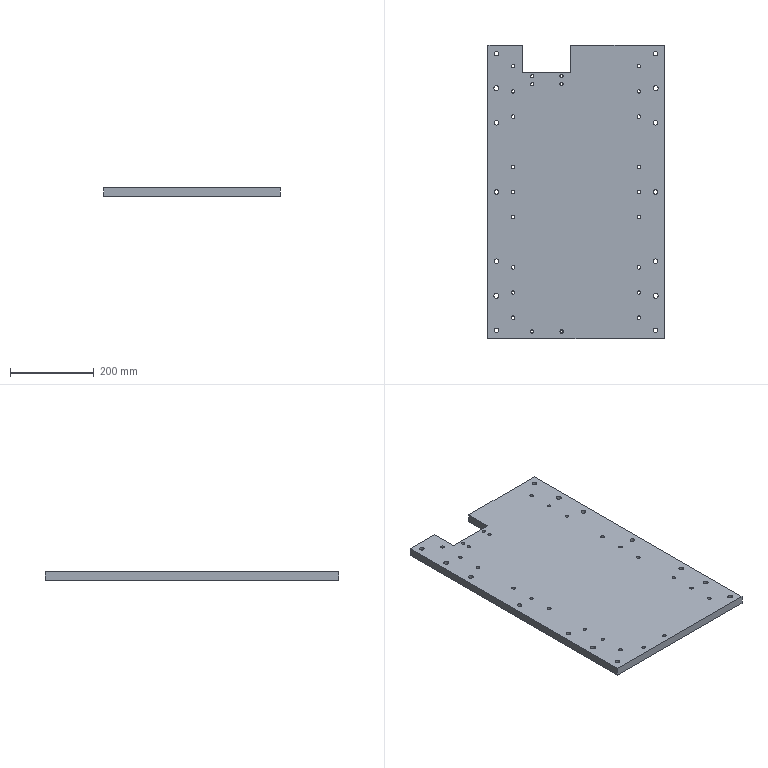Part | STEP file | Tube feed_id1166_x_t | 1 solid | 84 faces | box 420 x 700 x 19.5 mm | volume 5525930 mm3 | cylinder 50 | plane 22 | cone 12 | commonest cylinder face diameters 8.5 x12 14 x12 11 x10 6.8 x6 8 x6 12 x4